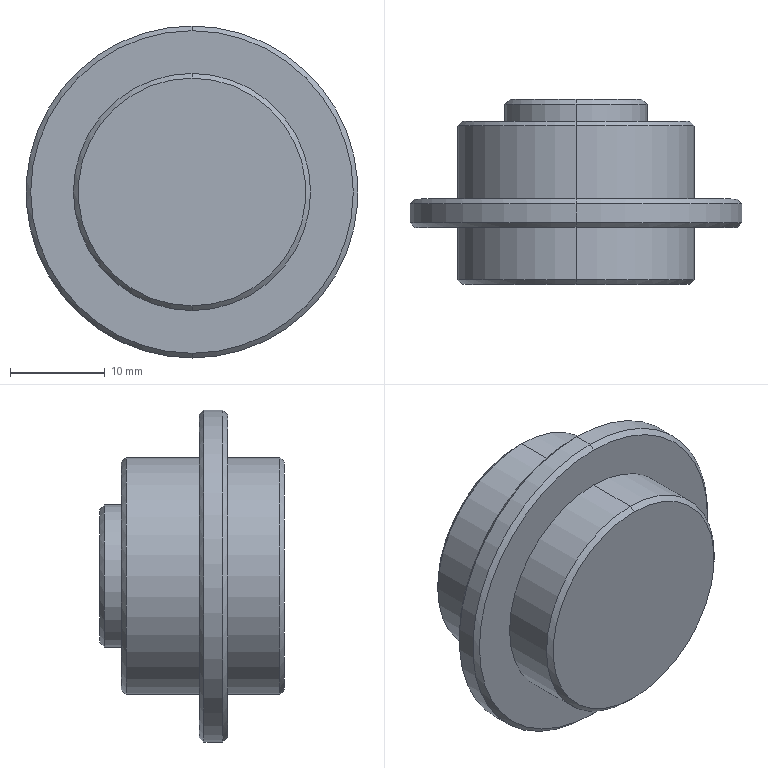Part | SolidWorks | features Chamfer 1, Revolution 1 | 1 solid | 23 faces | box 35 x 19.5 x 35 mm | volume 10211 mm3 | cone 10 | cylinder 8 | plane 5 | commonest cylinder face diameters 25 x4 15 x2 35 x2
STEP:
#1=CARTESIAN_POINT('',(368.,10.3,7.));
#2=VERTEX_POINT('',#1);
#3=CARTESIAN_POINT('',(368.,10.3,-7.));
#4=VERTEX_POINT('',#3);
#5=CARTESIAN_POINT('',(368.,10.3,0.));
#6=DIRECTION('',(0.,1.,0.));
#7=DIRECTION('',(0.,0.,-1.));
#8=AXIS2_PLACEMENT_3D('',#5,#6,#7);
#9=CIRCLE('',#8,7.);
#10=EDGE_CURVE('',#2,#4,#9,.T.);
#11=ORIENTED_EDGE('',*,*,#10,.F.);
#12=CARTESIAN_POINT('',(368.,9.8,7.5));
#13=VERTEX_POINT('',#12);
#14=CARTESIAN_POINT('',(368.,10.3,7.));
#15=DIRECTION('',(0.,-0.7071,0.7071));
#16=VECTOR('',#15,1000.);
#17=LINE('',#14,#16);
#18=EDGE_CURVE('',#2,#13,#17,.T.);
#19=ORIENTED_EDGE('',*,*,#18,.T.);
#20=CARTESIAN_POINT('',(368.,9.8,-7.5));
#21=VERTEX_POINT('',#20);
#22=CARTESIAN_POINT('',(368.,9.8,0.));
#23=DIRECTION('',(0.,-1.,0.));
#24=DIRECTION('',(0.,0.,-1.));
#25=AXIS2_PLACEMENT_3D('',#22,#23,#24);
#26=CIRCLE('',#25,7.5);
#27=EDGE_CURVE('',#21,#13,#26,.T.);
#28=ORIENTED_EDGE('',*,*,#27,.F.);
#29=CARTESIAN_POINT('',(368.,10.3,-7.));
#30=DIRECTION('',(0.,-0.7071,-0.7071));
#31=VECTOR('',#30,1000.);
#32=LINE('',#29,#31);
#33=EDGE_CURVE('',#4,#21,#32,.T.);
#34=ORIENTED_EDGE('',*,*,#33,.F.);
#35=EDGE_LOOP('',(#11,#19,#28,#34));
#36=FACE_OUTER_BOUND('',#35,.T.);
#37=CARTESIAN_POINT('',(368.,10.3,0.));
#38=DIRECTION('',(0.,-1.,0.));
#39=DIRECTION('',(0.,0.,-1.));
#40=AXIS2_PLACEMENT_3D('',#37,#38,#39);
#41=CONICAL_SURFACE('',#40,7.,0.7854);
#42=ADVANCED_FACE('',(#36),#41,.T.);
#43=CARTESIAN_POINT('',(368.,8.,12.));
#44=VERTEX_POINT('',#43);
#45=CARTESIAN_POINT('',(368.,8.,-12.));
#46=VERTEX_POINT('',#45);
#47=CARTESIAN_POINT('',(368.,8.,0.));
#48=DIRECTION('',(0.,1.,0.));
#49=DIRECTION('',(0.,0.,-1.));
#50=AXIS2_PLACEMENT_3D('',#47,#48,#49);
#51=CIRCLE('',#50,12.);
#52=EDGE_CURVE('',#44,#46,#51,.T.);
#53=ORIENTED_EDGE('',*,*,#52,.F.);
#54=CARTESIAN_POINT('',(368.,7.5,12.5));
#55=VERTEX_POINT('',#54);
#56=CARTESIAN_POINT('',(368.,8.,12.));
#57=DIRECTION('',(0.,-0.7071,0.7071));
#58=VECTOR('',#57,1000.);
#59=LINE('',#56,#58);
#60=EDGE_CURVE('',#44,#55,#59,.T.);
#61=ORIENTED_EDGE('',*,*,#60,.T.);
#62=CARTESIAN_POINT('',(368.,7.5,-12.5));
#63=VERTEX_POINT('',#62);
#64=CARTESIAN_POINT('',(368.,7.5,0.));
#65=DIRECTION('',(0.,-1.,0.));
#66=DIRECTION('',(0.,0.,-1.));
#67=AXIS2_PLACEMENT_3D('',#64,#65,#66);
#68=CIRCLE('',#67,12.5);
#69=EDGE_CURVE('',#63,#55,#68,.T.);
#70=ORIENTED_EDGE('',*,*,#69,.F.);
#71=CARTESIAN_POINT('',(368.,8.,-12.));
#72=DIRECTION('',(0.,-0.7071,-0.7071));
#73=VECTOR('',#72,1000.);
#74=LINE('',#71,#73);
#75=EDGE_CURVE('',#46,#63,#74,.T.);
#76=ORIENTED_EDGE('',*,*,#75,.F.);
#77=EDGE_LOOP('',(#53,#61,#70,#76));
#78=FACE_OUTER_BOUND('',#77,.T.);
#79=CARTESIAN_POINT('',(368.,8.,0.));
#80=DIRECTION('',(0.,-1.,0.));
#81=DIRECTION('',(0.,0.,-1.));
#82=AXIS2_PLACEMENT_3D('',#79,#80,#81);
#83=CONICAL_SURFACE('',#82,12.,0.7854);
#84=ADVANCED_FACE('',(#78),#83,.T.);
#85=CARTESIAN_POINT('',(368.,-0.2,17.));
#86=VERTEX_POINT('',#85);
#87=CARTESIAN_POINT('',(368.,-0.2,-17.));
#88=VERTEX_POINT('',#87);
#89=CARTESIAN_POINT('',(368.,-0.2,0.));
#90=DIRECTION('',(0.,1.,0.));
#91=DIRECTION('',(0.,0.,-1.));
#92=AXIS2_PLACEMENT_3D('',#89,#90,#91);
#93=CIRCLE('',#92,17.);
#94=EDGE_CURVE('',#86,#88,#93,.T.);
#95=ORIENTED_EDGE('',*,*,#94,.F.);
#96=CARTESIAN_POINT('',(368.,-0.7,17.5));
#97=VERTEX_POINT('',#96);
#98=CARTESIAN_POINT('',(368.,-0.2,17.));
#99=DIRECTION('',(0.,-0.7071,0.7071));
#100=VECTOR('',#99,1000.);
#101=LINE('',#98,#100);
#102=EDGE_CURVE('',#86,#97,#101,.T.);
#103=ORIENTED_EDGE('',*,*,#102,.T.);
#104=CARTESIAN_POINT('',(368.,-0.7,-17.5));
#105=VERTEX_POINT('',#104);
#106=CARTESIAN_POINT('',(368.,-0.7,0.));
#107=DIRECTION('',(0.,-1.,0.));
#108=DIRECTION('',(0.,0.,-1.));
#109=AXIS2_PLACEMENT_3D('',#106,#107,#108);
#110=CIRCLE('',#109,17.5);
#111=EDGE_CURVE('',#105,#97,#110,.T.);
#112=ORIENTED_EDGE('',*,*,#111,.F.);
#113=CARTESIAN_POINT('',(368.,-0.2,-17.));
#114=DIRECTION('',(0.,-0.7071,-0.7071));
#115=VECTOR('',#114,1000.);
#116=LINE('',#113,#115);
#117=EDGE_CURVE('',#88,#105,#116,.T.);
#118=ORIENTED_EDGE('',*,*,#117,.F.);
#119=EDGE_LOOP('',(#95,#103,#112,#118));
#120=FACE_OUTER_BOUND('',#119,.T.);
#121=CARTESIAN_POINT('',(368.,-0.2,0.));
#122=DIRECTION('',(0.,-1.,0.));
#123=DIRECTION('',(0.,0.,-1.));
#124=AXIS2_PLACEMENT_3D('',#121,#122,#123);
#125=CONICAL_SURFACE('',#124,17.,0.7854);
#126=ADVANCED_FACE('',(#120),#125,.T.);
#127=CARTESIAN_POINT('',(368.,-3.2,-17.));
#128=VERTEX_POINT('',#127);
#129=CARTESIAN_POINT('',(368.,-3.2,17.));
#130=VERTEX_POINT('',#129);
#131=CARTESIAN_POINT('',(368.,-3.2,0.));
#132=DIRECTION('',(0.,-1.,0.));
#133=DIRECTION('',(0.,0.,1.));
#134=AXIS2_PLACEMENT_3D('',#131,#132,#133);
#135=CIRCLE('',#134,17.);
#136=EDGE_CURVE('',#128,#130,#135,.T.);
#137=ORIENTED_EDGE('',*,*,#136,.F.);
#138=CARTESIAN_POINT('',(368.,-2.7,-17.5));
#139=VERTEX_POINT('',#138);
#140=CARTESIAN_POINT('',(368.,-2.7,-17.5));
#141=DIRECTION('',(0.,0.7071,-0.7071));
#142=VECTOR('',#141,1000.);
#143=LINE('',#140,#142);
#144=EDGE_CURVE('',#128,#139,#143,.T.);
#145=ORIENTED_EDGE('',*,*,#144,.T.);
#146=CARTESIAN_POINT('',(368.,-2.7,17.5));
#147=VERTEX_POINT('',#146);
#148=CARTESIAN_POINT('',(368.,-2.7,0.));
#149=DIRECTION('',(0.,1.,0.));
#150=DIRECTION('',(0.,0.,1.));
#151=AXIS2_PLACEMENT_3D('',#148,#149,#150);
#152=CIRCLE('',#151,17.5);
#153=EDGE_CURVE('',#147,#139,#152,.T.);
#154=ORIENTED_EDGE('',*,*,#153,.F.);
#155=CARTESIAN_POINT('',(368.,-2.7,17.5));
#156=DIRECTION('',(0.,0.7071,0.7071));
#157=VECTOR('',#156,1000.);
#158=LINE('',#155,#157);
#159=EDGE_CURVE('',#130,#147,#158,.T.);
#160=ORIENTED_EDGE('',*,*,#159,.F.);
#161=EDGE_LOOP('',(#137,#145,#154,#160));
#162=FACE_OUTER_BOUND('',#161,.T.);
#163=CARTESIAN_POINT('',(368.,-2.7,0.));
#164=DIRECTION('',(0.,1.,0.));
#165=DIRECTION('',(0.,0.,1.));
#166=AXIS2_PLACEMENT_3D('',#163,#164,#165);
#167=CONICAL_SURFACE('',#166,17.5,0.7854);
#168=ADVANCED_FACE('',(#162),#167,.T.);
#169=CARTESIAN_POINT('',(368.,-9.2,-12.));
#170=VERTEX_POINT('',#169);
#171=CARTESIAN_POINT('',(368.,-9.2,12.));
#172=VERTEX_POINT('',#171);
#173=CARTESIAN_POINT('',(368.,-9.2,0.));
#174=DIRECTION('',(0.,-1.,0.));
#175=DIRECTION('',(0.,0.,1.));
#176=AXIS2_PLACEMENT_3D('',#173,#174,#175);
#177=CIRCLE('',#176,12.);
#178=EDGE_CURVE('',#170,#172,#177,.T.);
#179=ORIENTED_EDGE('',*,*,#178,.F.);
#180=CARTESIAN_POINT('',(368.,-8.7,-12.5));
#181=VERTEX_POINT('',#180);
#182=CARTESIAN_POINT('',(368.,-8.7,-12.5));
#183=DIRECTION('',(0.,0.7071,-0.7071));
#184=VECTOR('',#183,1000.);
#185=LINE('',#182,#184);
#186=EDGE_CURVE('',#170,#181,#185,.T.);
#187=ORIENTED_EDGE('',*,*,#186,.T.);
#188=CARTESIAN_POINT('',(368.,-8.7,12.5));
#189=VERTEX_POINT('',#188);
#190=CARTESIAN_POINT('',(368.,-8.7,0.));
#191=DIRECTION('',(0.,1.,0.));
#192=DIRECTION('',(0.,0.,1.));
#193=AXIS2_PLACEMENT_3D('',#190,#191,#192);
#194=CIRCLE('',#193,12.5);
#195=EDGE_CURVE('',#189,#181,#194,.T.);
#196=ORIENTED_EDGE('',*,*,#195,.F.);
#197=CARTESIAN_POINT('',(368.,-8.7,12.5));
#198=DIRECTION('',(0.,0.7071,0.7071));
#199=VECTOR('',#198,1000.);
#200=LINE('',#197,#199);
#201=EDGE_CURVE('',#172,#189,#200,.T.);
#202=ORIENTED_EDGE('',*,*,#201,.F.);
#203=EDGE_LOOP('',(#179,#187,#196,#202));
#204=FACE_OUTER_BOUND('',#203,.T.);
#205=CARTESIAN_POINT('',(368.,-8.7,0.));
#206=DIRECTION('',(0.,1.,0.));
#207=DIRECTION('',(0.,0.,1.));
#208=AXIS2_PLACEMENT_3D('',#205,#206,#207);
#209=CONICAL_SURFACE('',#208,12.5,0.7854);
#210=ADVANCED_FACE('',(#204),#209,.T.);
#211=CARTESIAN_POINT('',(368.,8.,7.5));
#212=VERTEX_POINT('',#211);
#213=CARTESIAN_POINT('',(368.,8.,-7.5));
#214=VERTEX_POINT('',#213);
#215=CARTESIAN_POINT('',(368.,8.,0.));
#216=DIRECTION('',(0.,1.,0.));
#217=DIRECTION('',(0.,0.,1.));
#218=AXIS2_PLACEMENT_3D('',#215,#216,#217);
#219=CIRCLE('',#218,7.5);
#220=EDGE_CURVE('',#212,#214,#219,.T.);
#221=ORIENTED_EDGE('',*,*,#220,.T.);
#222=CARTESIAN_POINT('',(368.,10.3,-7.5));
#223=DIRECTION('',(0.,1.,0.));
#224=VECTOR('',#223,1000.);
#225=LINE('',#222,#224);
#226=EDGE_CURVE('',#214,#21,#225,.T.);
#227=ORIENTED_EDGE('',*,*,#226,.T.);
#228=ORIENTED_EDGE('',*,*,#27,.T.);
#229=CARTESIAN_POINT('',(368.,10.3,7.5));
#230=DIRECTION('',(0.,1.,0.));
#231=VECTOR('',#230,1000.);
#232=LINE('',#229,#231);
#233=EDGE_CURVE('',#212,#13,#232,.T.);
#234=ORIENTED_EDGE('',*,*,#233,.F.);
#235=EDGE_LOOP('',(#221,#227,#228,#234));
#236=FACE_OUTER_BOUND('',#235,.T.);
#237=CARTESIAN_POINT('',(368.,10.3,0.));
#238=DIRECTION('',(0.,1.,0.));
#239=DIRECTION('',(0.,0.,1.));
#240=AXIS2_PLACEMENT_3D('',#237,#238,#239);
#241=CYLINDRICAL_SURFACE('',#240,7.5);
#242=ADVANCED_FACE('',(#236),#241,.T.);
#243=CARTESIAN_POINT('',(368.,-0.2,12.5));
#244=VERTEX_POINT('',#243);
#245=CARTESIAN_POINT('',(368.,-0.2,-12.5));
#246=VERTEX_POINT('',#245);
#247=CARTESIAN_POINT('',(368.,-0.2,0.));
#248=DIRECTION('',(0.,1.,0.));
#249=DIRECTION('',(0.,0.,1.));
#250=AXIS2_PLACEMENT_3D('',#247,#248,#249);
#251=CIRCLE('',#250,12.5);
#252=EDGE_CURVE('',#244,#246,#251,.T.);
#253=ORIENTED_EDGE('',*,*,#252,.T.);
#254=CARTESIAN_POINT('',(368.,10.3,-12.5));
#255=DIRECTION('',(0.,1.,0.));
#256=VECTOR('',#255,1000.);
#257=LINE('',#254,#256);
#258=EDGE_CURVE('',#246,#63,#257,.T.);
#259=ORIENTED_EDGE('',*,*,#258,.T.);
#260=ORIENTED_EDGE('',*,*,#69,.T.);
#261=CARTESIAN_POINT('',(368.,10.3,12.5));
#262=DIRECTION('',(0.,1.,0.));
#263=VECTOR('',#262,1000.);
#264=LINE('',#261,#263);
#265=EDGE_CURVE('',#244,#55,#264,.T.);
#266=ORIENTED_EDGE('',*,*,#265,.F.);
#267=EDGE_LOOP('',(#253,#259,#260,#266));
#268=FACE_OUTER_BOUND('',#267,.T.);
#269=CARTESIAN_POINT('',(368.,10.3,0.));
#270=DIRECTION('',(0.,1.,0.));
#271=DIRECTION('',(0.,0.,1.));
#272=AXIS2_PLACEMENT_3D('',#269,#270,#271);
#273=CYLINDRICAL_SURFACE('',#272,12.5);
#274=ADVANCED_FACE('',(#268),#273,.T.);
#275=ORIENTED_EDGE('',*,*,#153,.T.);
#276=CARTESIAN_POINT('',(368.,10.3,-17.5));
#277=DIRECTION('',(0.,1.,0.));
#278=VECTOR('',#277,1000.);
#279=LINE('',#276,#278);
#280=EDGE_CURVE('',#139,#105,#279,.T.);
#281=ORIENTED_EDGE('',*,*,#280,.T.);
#282=ORIENTED_EDGE('',*,*,#111,.T.);
#283=CARTESIAN_POINT('',(368.,10.3,17.5));
#284=DIRECTION('',(0.,1.,0.));
#285=VECTOR('',#284,1000.);
#286=LINE('',#283,#285);
#287=EDGE_CURVE('',#147,#97,#286,.T.);
#288=ORIENTED_EDGE('',*,*,#287,.F.);
#289=EDGE_LOOP('',(#275,#281,#282,#288));
#290=FACE_OUTER_BOUND('',#289,.T.);
#291=CARTESIAN_POINT('',(368.,10.3,0.));
#292=DIRECTION('',(0.,1.,0.));
#293=DIRECTION('',(0.,0.,1.));
#294=AXIS2_PLACEMENT_3D('',#291,#292,#293);
#295=CYLINDRICAL_SURFACE('',#294,17.5);
#296=ADVANCED_FACE('',(#290),#295,.T.);
#297=ORIENTED_EDGE('',*,*,#195,.T.);
#298=CARTESIAN_POINT('',(368.,-3.2,-12.5));
#299=VERTEX_POINT('',#298);
#300=CARTESIAN_POINT('',(368.,10.3,-12.5));
#301=DIRECTION('',(0.,1.,0.));
#302=VECTOR('',#301,1000.);
#303=LINE('',#300,#302);
#304=EDGE_CURVE('',#181,#299,#303,.T.);
#305=ORIENTED_EDGE('',*,*,#304,.T.);
#306=CARTESIAN_POINT('',(368.,-3.2,12.5));
#307=VERTEX_POINT('',#306);
#308=CARTESIAN_POINT('',(368.,-3.2,0.));
#309=DIRECTION('',(0.,1.,0.));
#310=DIRECTION('',(0.,0.,1.));
#311=AXIS2_PLACEMENT_3D('',#308,#309,#310);
#312=CIRCLE('',#311,12.5);
#313=EDGE_CURVE('',#307,#299,#312,.T.);
#314=ORIENTED_EDGE('',*,*,#313,.F.);
#315=CARTESIAN_POINT('',(368.,10.3,12.5));
#316=DIRECTION('',(0.,1.,0.));
#317=VECTOR('',#316,1000.);
#318=LINE('',#315,#317);
#319=EDGE_CURVE('',#189,#307,#318,.T.);
#320=ORIENTED_EDGE('',*,*,#319,.F.);
#321=EDGE_LOOP('',(#297,#305,#314,#320));
#322=FACE_OUTER_BOUND('',#321,.T.);
#323=CARTESIAN_POINT('',(368.,10.3,0.));
#324=DIRECTION('',(0.,1.,0.));
#325=DIRECTION('',(0.,0.,1.));
#326=AXIS2_PLACEMENT_3D('',#323,#324,#325);
#327=CYLINDRICAL_SURFACE('',#326,12.5);
#328=ADVANCED_FACE('',(#322),#327,.T.);
#329=CARTESIAN_POINT('',(368.,-9.2,0.));
#330=DIRECTION('',(0.,-1.,0.));
#331=DIRECTION('',(0.,0.,1.));
#332=AXIS2_PLACEMENT_3D('',#329,#330,#331);
#333=CIRCLE('',#332,12.);
#334=EDGE_CURVE('',#172,#170,#333,.T.);
#335=ORIENTED_EDGE('',*,*,#334,.T.);
#336=ORIENTED_EDGE('',*,*,#178,.T.);
#337=EDGE_LOOP('',(#335,#336));
#338=FACE_OUTER_BOUND('',#337,.T.);
#339=CARTESIAN_POINT('',(380.5,-9.2,0.));
#340=DIRECTION('',(0.,1.,0.));
#341=DIRECTION('',(0.,0.,1.));
#342=AXIS2_PLACEMENT_3D('',#339,#340,#341);
#343=PLANE('',#342);
#344=ADVANCED_FACE('',(#338),#343,.F.);
#345=ORIENTED_EDGE('',*,*,#304,.F.);
#346=CARTESIAN_POINT('',(368.,-8.7,0.));
#347=DIRECTION('',(0.,1.,0.));
#348=DIRECTION('',(0.,0.,1.));
#349=AXIS2_PLACEMENT_3D('',#346,#347,#348);
#350=CIRCLE('',#349,12.5);
#351=EDGE_CURVE('',#181,#189,#350,.T.);
#352=ORIENTED_EDGE('',*,*,#351,.T.);
#353=ORIENTED_EDGE('',*,*,#319,.T.);
#354=CARTESIAN_POINT('',(368.,-3.2,0.));
#355=DIRECTION('',(0.,1.,0.));
#356=DIRECTION('',(0.,0.,1.));
#357=AXIS2_PLACEMENT_3D('',#354,#355,#356);
#358=CIRCLE('',#357,12.5);
#359=EDGE_CURVE('',#299,#307,#358,.T.);
#360=ORIENTED_EDGE('',*,*,#359,.F.);
#361=EDGE_LOOP('',(#345,#352,#353,#360));
#362=FACE_OUTER_BOUND('',#361,.T.);
#363=CARTESIAN_POINT('',(368.,10.3,0.));
#364=DIRECTION('',(0.,1.,0.));
#365=DIRECTION('',(0.,0.,1.));
#366=AXIS2_PLACEMENT_3D('',#363,#364,#365);
#367=CYLINDRICAL_SURFACE('',#366,12.5);
#368=ADVANCED_FACE('',(#362),#367,.T.);
#369=CARTESIAN_POINT('',(368.,-3.2,0.));
#370=DIRECTION('',(0.,-1.,0.));
#371=DIRECTION('',(0.,0.,1.));
#372=AXIS2_PLACEMENT_3D('',#369,#370,#371);
#373=CIRCLE('',#372,17.);
#374=EDGE_CURVE('',#130,#128,#373,.T.);
#375=ORIENTED_EDGE('',*,*,#374,.T.);
#376=ORIENTED_EDGE('',*,*,#136,.T.);
#377=EDGE_LOOP('',(#375,#376));
#378=FACE_OUTER_BOUND('',#377,.T.);
#379=ORIENTED_EDGE('',*,*,#313,.T.);
#380=ORIENTED_EDGE('',*,*,#359,.T.);
#381=EDGE_LOOP('',(#379,#380));
#382=FACE_BOUND('',#381,.T.);
#383=CARTESIAN_POINT('',(380.5,-3.2,0.));
#384=DIRECTION('',(0.,1.,0.));
#385=DIRECTION('',(0.,0.,1.));
#386=AXIS2_PLACEMENT_3D('',#383,#384,#385);
#387=PLANE('',#386);
#388=ADVANCED_FACE('',(#378,#382),#387,.F.);
#389=ORIENTED_EDGE('',*,*,#280,.F.);
#390=CARTESIAN_POINT('',(368.,-2.7,0.));
#391=DIRECTION('',(0.,1.,0.));
#392=DIRECTION('',(0.,0.,1.));
#393=AXIS2_PLACEMENT_3D('',#390,#391,#392);
#394=CIRCLE('',#393,17.5);
#395=EDGE_CURVE('',#139,#147,#394,.T.);
#396=ORIENTED_EDGE('',*,*,#395,.T.);
#397=ORIENTED_EDGE('',*,*,#287,.T.);
#398=CARTESIAN_POINT('',(368.,-0.7,0.));
#399=DIRECTION('',(0.,-1.,0.));
#400=DIRECTION('',(0.,0.,-1.));
#401=AXIS2_PLACEMENT_3D('',#398,#399,#400);
#402=CIRCLE('',#401,17.5);
#403=EDGE_CURVE('',#97,#105,#402,.T.);
#404=ORIENTED_EDGE('',*,*,#403,.T.);
#405=EDGE_LOOP('',(#389,#396,#397,#404));
#406=FACE_OUTER_BOUND('',#405,.T.);
#407=CARTESIAN_POINT('',(368.,10.3,0.));
#408=DIRECTION('',(0.,1.,0.));
#409=DIRECTION('',(0.,0.,1.));
#410=AXIS2_PLACEMENT_3D('',#407,#408,#409);
#411=CYLINDRICAL_SURFACE('',#410,17.5);
#412=ADVANCED_FACE('',(#406),#411,.T.);
#413=CARTESIAN_POINT('',(368.,-0.2,0.));
#414=DIRECTION('',(0.,1.,0.));
#415=DIRECTION('',(0.,0.,-1.));
#416=AXIS2_PLACEMENT_3D('',#413,#414,#415);
#417=CIRCLE('',#416,17.);
#418=EDGE_CURVE('',#88,#86,#417,.T.);
#419=ORIENTED_EDGE('',*,*,#418,.T.);
#420=ORIENTED_EDGE('',*,*,#94,.T.);
#421=EDGE_LOOP('',(#419,#420));
#422=FACE_OUTER_BOUND('',#421,.T.);
#423=ORIENTED_EDGE('',*,*,#252,.F.);
#424=CARTESIAN_POINT('',(368.,-0.2,0.));
#425=DIRECTION('',(0.,1.,0.));
#426=DIRECTION('',(0.,0.,1.));
#427=AXIS2_PLACEMENT_3D('',#424,#425,#426);
#428=CIRCLE('',#427,12.5);
#429=EDGE_CURVE('',#246,#244,#428,.T.);
#430=ORIENTED_EDGE('',*,*,#429,.F.);
#431=EDGE_LOOP('',(#423,#430));
#432=FACE_BOUND('',#431,.T.);
#433=CARTESIAN_POINT('',(385.5,-0.2,0.));
#434=DIRECTION('',(0.,-1.,0.));
#435=DIRECTION('',(0.,0.,-1.));
#436=AXIS2_PLACEMENT_3D('',#433,#434,#435);
#437=PLANE('',#436);
#438=ADVANCED_FACE('',(#422,#432),#437,.F.);
#439=ORIENTED_EDGE('',*,*,#258,.F.);
#440=ORIENTED_EDGE('',*,*,#429,.T.);
#441=ORIENTED_EDGE('',*,*,#265,.T.);
#442=CARTESIAN_POINT('',(368.,7.5,0.));
#443=DIRECTION('',(0.,-1.,0.));
#444=DIRECTION('',(0.,0.,-1.));
#445=AXIS2_PLACEMENT_3D('',#442,#443,#444);
#446=CIRCLE('',#445,12.5);
#447=EDGE_CURVE('',#55,#63,#446,.T.);
#448=ORIENTED_EDGE('',*,*,#447,.T.);
#449=EDGE_LOOP('',(#439,#440,#441,#448));
#450=FACE_OUTER_BOUND('',#449,.T.);
#451=CARTESIAN_POINT('',(368.,10.3,0.));
#452=DIRECTION('',(0.,1.,0.));
#453=DIRECTION('',(0.,0.,1.));
#454=AXIS2_PLACEMENT_3D('',#451,#452,#453);
#455=CYLINDRICAL_SURFACE('',#454,12.5);
#456=ADVANCED_FACE('',(#450),#455,.T.);
#457=CARTESIAN_POINT('',(368.,8.,0.));
#458=DIRECTION('',(0.,1.,0.));
#459=DIRECTION('',(0.,0.,-1.));
#460=AXIS2_PLACEMENT_3D('',#457,#458,#459);
#461=CIRCLE('',#460,12.);
#462=EDGE_CURVE('',#46,#44,#461,.T.);
#463=ORIENTED_EDGE('',*,*,#462,.T.);
#464=ORIENTED_EDGE('',*,*,#52,.T.);
#465=EDGE_LOOP('',(#463,#464));
#466=FACE_OUTER_BOUND('',#465,.T.);
#467=ORIENTED_EDGE('',*,*,#220,.F.);
#468=CARTESIAN_POINT('',(368.,8.,0.));
#469=DIRECTION('',(0.,1.,0.));
#470=DIRECTION('',(0.,0.,1.));
#471=AXIS2_PLACEMENT_3D('',#468,#469,#470);
#472=CIRCLE('',#471,7.5);
#473=EDGE_CURVE('',#214,#212,#472,.T.);
#474=ORIENTED_EDGE('',*,*,#473,.F.);
#475=EDGE_LOOP('',(#467,#474));
#476=FACE_BOUND('',#475,.T.);
#477=CARTESIAN_POINT('',(380.5,8.,0.));
#478=DIRECTION('',(0.,-1.,0.));
#479=DIRECTION('',(0.,0.,-1.));
#480=AXIS2_PLACEMENT_3D('',#477,#478,#479);
#481=PLANE('',#480);
#482=ADVANCED_FACE('',(#466,#476),#481,.F.);
#483=ORIENTED_EDGE('',*,*,#226,.F.);
#484=ORIENTED_EDGE('',*,*,#473,.T.);
#485=ORIENTED_EDGE('',*,*,#233,.T.);
#486=CARTESIAN_POINT('',(368.,9.8,0.));
#487=DIRECTION('',(0.,-1.,0.));
#488=DIRECTION('',(0.,0.,-1.));
#489=AXIS2_PLACEMENT_3D('',#486,#487,#488);
#490=CIRCLE('',#489,7.5);
#491=EDGE_CURVE('',#13,#21,#490,.T.);
#492=ORIENTED_EDGE('',*,*,#491,.T.);
#493=EDGE_LOOP('',(#483,#484,#485,#492));
#494=FACE_OUTER_BOUND('',#493,.T.);
#495=CARTESIAN_POINT('',(368.,10.3,0.));
#496=DIRECTION('',(0.,1.,0.));
#497=DIRECTION('',(0.,0.,1.));
#498=AXIS2_PLACEMENT_3D('',#495,#496,#497);
#499=CYLINDRICAL_SURFACE('',#498,7.5);
#500=ADVANCED_FACE('',(#494),#499,.T.);
#501=CARTESIAN_POINT('',(368.,10.3,0.));
#502=DIRECTION('',(0.,1.,0.));
#503=DIRECTION('',(0.,0.,-1.));
#504=AXIS2_PLACEMENT_3D('',#501,#502,#503);
#505=CIRCLE('',#504,7.);
#506=EDGE_CURVE('',#4,#2,#505,.T.);
#507=ORIENTED_EDGE('',*,*,#506,.T.);
#508=ORIENTED_EDGE('',*,*,#10,.T.);
#509=EDGE_LOOP('',(#507,#508));
#510=FACE_OUTER_BOUND('',#509,.T.);
#511=CARTESIAN_POINT('',(375.5,10.3,0.));
#512=DIRECTION('',(0.,-1.,0.));
#513=DIRECTION('',(0.,0.,-1.));
#514=AXIS2_PLACEMENT_3D('',#511,#512,#513);
#515=PLANE('',#514);
#516=ADVANCED_FACE('',(#510),#515,.F.);
#517=ORIENTED_EDGE('',*,*,#186,.F.);
#518=ORIENTED_EDGE('',*,*,#334,.F.);
#519=ORIENTED_EDGE('',*,*,#201,.T.);
#520=ORIENTED_EDGE('',*,*,#351,.F.);
#521=EDGE_LOOP('',(#517,#518,#519,#520));
#522=FACE_OUTER_BOUND('',#521,.T.);
#523=CARTESIAN_POINT('',(368.,-8.7,0.));
#524=DIRECTION('',(0.,1.,0.));
#525=DIRECTION('',(0.,0.,1.));
#526=AXIS2_PLACEMENT_3D('',#523,#524,#525);
#527=CONICAL_SURFACE('',#526,12.5,0.7854);
#528=ADVANCED_FACE('',(#522),#527,.T.);
#529=ORIENTED_EDGE('',*,*,#144,.F.);
#530=ORIENTED_EDGE('',*,*,#374,.F.);
#531=ORIENTED_EDGE('',*,*,#159,.T.);
#532=ORIENTED_EDGE('',*,*,#395,.F.);
#533=EDGE_LOOP('',(#529,#530,#531,#532));
#534=FACE_OUTER_BOUND('',#533,.T.);
#535=CARTESIAN_POINT('',(368.,-2.7,0.));
#536=DIRECTION('',(0.,1.,0.));
#537=DIRECTION('',(0.,0.,1.));
#538=AXIS2_PLACEMENT_3D('',#535,#536,#537);
#539=CONICAL_SURFACE('',#538,17.5,0.7854);
#540=ADVANCED_FACE('',(#534),#539,.T.);
#541=ORIENTED_EDGE('',*,*,#102,.F.);
#542=ORIENTED_EDGE('',*,*,#418,.F.);
#543=ORIENTED_EDGE('',*,*,#117,.T.);
#544=ORIENTED_EDGE('',*,*,#403,.F.);
#545=EDGE_LOOP('',(#541,#542,#543,#544));
#546=FACE_OUTER_BOUND('',#545,.T.);
#547=CARTESIAN_POINT('',(368.,-0.2,0.));
#548=DIRECTION('',(0.,-1.,0.));
#549=DIRECTION('',(0.,0.,-1.));
#550=AXIS2_PLACEMENT_3D('',#547,#548,#549);
#551=CONICAL_SURFACE('',#550,17.,0.7854);
#552=ADVANCED_FACE('',(#546),#551,.T.);
#553=ORIENTED_EDGE('',*,*,#60,.F.);
#554=ORIENTED_EDGE('',*,*,#462,.F.);
#555=ORIENTED_EDGE('',*,*,#75,.T.);
#556=ORIENTED_EDGE('',*,*,#447,.F.);
#557=EDGE_LOOP('',(#553,#554,#555,#556));
#558=FACE_OUTER_BOUND('',#557,.T.);
#559=CARTESIAN_POINT('',(368.,8.,0.));
#560=DIRECTION('',(0.,-1.,0.));
#561=DIRECTION('',(0.,0.,-1.));
#562=AXIS2_PLACEMENT_3D('',#559,#560,#561);
#563=CONICAL_SURFACE('',#562,12.,0.7854);
#564=ADVANCED_FACE('',(#558),#563,.T.);
#565=ORIENTED_EDGE('',*,*,#18,.F.);
#566=ORIENTED_EDGE('',*,*,#506,.F.);
#567=ORIENTED_EDGE('',*,*,#33,.T.);
#568=ORIENTED_EDGE('',*,*,#491,.F.);
#569=EDGE_LOOP('',(#565,#566,#567,#568));
#570=FACE_OUTER_BOUND('',#569,.T.);
#571=CARTESIAN_POINT('',(368.,10.3,0.));
#572=DIRECTION('',(0.,-1.,0.));
#573=DIRECTION('',(0.,0.,-1.));
#574=AXIS2_PLACEMENT_3D('',#571,#572,#573);
#575=CONICAL_SURFACE('',#574,7.,0.7854);
#576=ADVANCED_FACE('',(#570),#575,.T.);
#577=CLOSED_SHELL('',(#42,#84,#126,#168,#210,#242,#274,#296,#328,#344,#368,#388,#412,#438,#456,#482,#500,#516,#528,#540,#552,#564,#576));
#578=MANIFOLD_SOLID_BREP('',#577);
#579=CARTESIAN_POINT('',(0.,0.,0.));
#580=DIRECTION('',(0.,0.,1.));
#581=DIRECTION('',(1.,0.,0.));
#582=AXIS2_PLACEMENT_3D('',#579,#580,#581);
#583=(LENGTH_UNIT()NAMED_UNIT(*)SI_UNIT(.MILLI.,.METRE.));
#584=UNCERTAINTY_MEASURE_WITH_UNIT(LENGTH_MEASURE(0.00001),#583,'','');
#585=(NAMED_UNIT(*)PLANE_ANGLE_UNIT()SI_UNIT($,.RADIAN.));
#586=(NAMED_UNIT(*)SI_UNIT($,.STERADIAN.)SOLID_ANGLE_UNIT());
#587=(GEOMETRIC_REPRESENTATION_CONTEXT(3)GLOBAL_UNCERTAINTY_ASSIGNED_CONTEXT((#584))GLOBAL_UNIT_ASSIGNED_CONTEXT((#583,#585,#586))REPRESENTATION_CONTEXT('',''));
#588=ADVANCED_BREP_SHAPE_REPRESENTATION('',(#578,#582),#587);